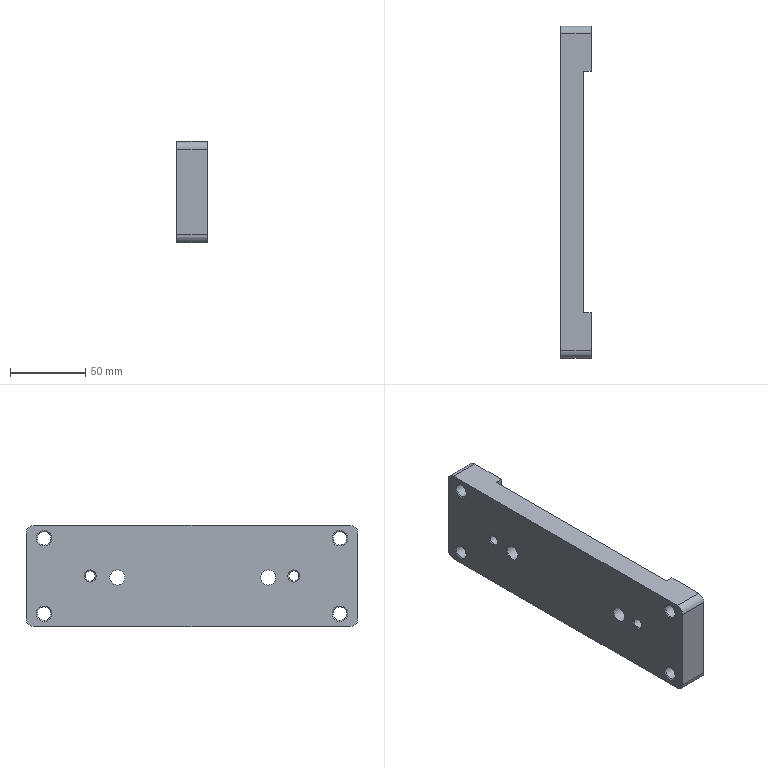Part | NX | features SIMPLE HOLE 8, DATUM_CSYS 6, SKETCH 5, HOLE PACKAGE 3, EXTRUDE 2, SYMBOLIC_THREAD 2, BLEND 1, LINKED_CURVE 1, LINKED_FACE 1 | 1 solid | 32 faces | box 20 x 220 x 67 mm | volume 232185 mm3 | cylinder 12 | plane 10 | cone 10 | commonest cylinder face diameters 10 x6 9 x4 6.8 x2
STEP:
#1=CARTESIAN_POINT('',(85.,105.,477.));
#2=VERTEX_POINT('',#1);
#3=CARTESIAN_POINT('',(85.,80.,477.));
#4=VERTEX_POINT('',#3);
#5=CARTESIAN_POINT('',(85.,110.,477.));
#6=DIRECTION('',(0.,-1.,0.));
#7=VECTOR('',#6,1000.);
#8=LINE('',#5,#7);
#9=EDGE_CURVE('',#2,#4,#8,.T.);
#10=ORIENTED_EDGE('',*,*,#9,.F.);
#11=CARTESIAN_POINT('',(65.,105.,477.));
#12=VERTEX_POINT('',#11);
#13=CARTESIAN_POINT('',(85.,105.,477.));
#14=DIRECTION('',(-1.,0.,0.));
#15=VECTOR('',#14,1000.);
#16=LINE('',#13,#15);
#17=EDGE_CURVE('',#2,#12,#16,.T.);
#18=ORIENTED_EDGE('',*,*,#17,.T.);
#19=CARTESIAN_POINT('',(65.,-105.,477.));
#20=VERTEX_POINT('',#19);
#21=CARTESIAN_POINT('',(65.,110.,477.));
#22=DIRECTION('',(0.,-1.,0.));
#23=VECTOR('',#22,1000.);
#24=LINE('',#21,#23);
#25=EDGE_CURVE('',#12,#20,#24,.T.);
#26=ORIENTED_EDGE('',*,*,#25,.T.);
#27=CARTESIAN_POINT('',(85.,-105.,477.));
#28=VERTEX_POINT('',#27);
#29=CARTESIAN_POINT('',(85.,-105.,477.));
#30=DIRECTION('',(-1.,0.,0.));
#31=VECTOR('',#30,1000.);
#32=LINE('',#29,#31);
#33=EDGE_CURVE('',#20,#28,#32,.F.);
#34=ORIENTED_EDGE('',*,*,#33,.T.);
#35=CARTESIAN_POINT('',(85.,-80.,477.));
#36=VERTEX_POINT('',#35);
#37=CARTESIAN_POINT('',(85.,110.,477.));
#38=DIRECTION('',(0.,-1.,0.));
#39=VECTOR('',#38,1000.);
#40=LINE('',#37,#39);
#41=EDGE_CURVE('',#36,#28,#40,.T.);
#42=ORIENTED_EDGE('',*,*,#41,.F.);
#43=CARTESIAN_POINT('',(80.,-80.,477.));
#44=VERTEX_POINT('',#43);
#45=CARTESIAN_POINT('',(80.,-80.,477.));
#46=DIRECTION('',(1.,0.,0.));
#47=VECTOR('',#46,1000.);
#48=LINE('',#45,#47);
#49=EDGE_CURVE('',#44,#36,#48,.T.);
#50=ORIENTED_EDGE('',*,*,#49,.F.);
#51=CARTESIAN_POINT('',(80.,80.,477.));
#52=VERTEX_POINT('',#51);
#53=CARTESIAN_POINT('',(80.,80.,477.));
#54=DIRECTION('',(0.,-1.,0.));
#55=VECTOR('',#54,1000.);
#56=LINE('',#53,#55);
#57=EDGE_CURVE('',#52,#44,#56,.T.);
#58=ORIENTED_EDGE('',*,*,#57,.F.);
#59=CARTESIAN_POINT('',(118.,80.,477.));
#60=DIRECTION('',(-1.,0.,0.));
#61=VECTOR('',#60,1000.);
#62=LINE('',#59,#61);
#63=EDGE_CURVE('',#4,#52,#62,.T.);
#64=ORIENTED_EDGE('',*,*,#63,.F.);
#65=EDGE_LOOP('',(#10,#18,#26,#34,#42,#50,#58,#64));
#66=FACE_BOUND('',#65,.T.);
#67=CARTESIAN_POINT('',(85.,110.,477.));
#68=DIRECTION('',(0.,0.,-1.));
#69=DIRECTION('',(0.,1.,0.));
#70=AXIS2_PLACEMENT_3D('',#67,#68,#69);
#71=PLANE('',#70);
#72=ADVANCED_FACE('',(#66),#71,.F.);
#73=CARTESIAN_POINT('',(85.,-98.,463.4));
#74=VERTEX_POINT('',#73);
#75=CARTESIAN_POINT('',(85.,-98.,468.5));
#76=DIRECTION('',(1.,0.,0.));
#77=DIRECTION('',(0.,0.,-1.));
#78=AXIS2_PLACEMENT_3D('',#75,#76,#77);
#79=CIRCLE('',#78,5.1);
#80=EDGE_CURVE('',#74,#74,#79,.F.);
#81=ORIENTED_EDGE('',*,*,#80,.T.);
#82=EDGE_LOOP('',(#81));
#83=FACE_BOUND('',#82,.T.);
#84=CARTESIAN_POINT('',(85.,-98.,413.4));
#85=VERTEX_POINT('',#84);
#86=CARTESIAN_POINT('',(85.,-98.,418.5));
#87=DIRECTION('',(1.,0.,0.));
#88=DIRECTION('',(0.,0.,-1.));
#89=AXIS2_PLACEMENT_3D('',#86,#87,#88);
#90=CIRCLE('',#89,5.1);
#91=EDGE_CURVE('',#85,#85,#90,.F.);
#92=ORIENTED_EDGE('',*,*,#91,.T.);
#93=EDGE_LOOP('',(#92));
#94=FACE_BOUND('',#93,.T.);
#95=CARTESIAN_POINT('',(85.,-110.,472.));
#96=VERTEX_POINT('',#95);
#97=CARTESIAN_POINT('',(85.,-110.,415.));
#98=VERTEX_POINT('',#97);
#99=CARTESIAN_POINT('',(85.,-110.,477.));
#100=DIRECTION('',(0.,0.,-1.));
#101=VECTOR('',#100,1000.);
#102=LINE('',#99,#101);
#103=EDGE_CURVE('',#96,#98,#102,.T.);
#104=ORIENTED_EDGE('',*,*,#103,.T.);
#105=CARTESIAN_POINT('',(85.,-105.,410.));
#106=VERTEX_POINT('',#105);
#107=CARTESIAN_POINT('',(85.,-105.,415.));
#108=DIRECTION('',(1.,0.,0.));
#109=DIRECTION('',(0.,0.,-1.));
#110=AXIS2_PLACEMENT_3D('',#107,#108,#109);
#111=CIRCLE('',#110,5.);
#112=EDGE_CURVE('',#98,#106,#111,.T.);
#113=ORIENTED_EDGE('',*,*,#112,.T.);
#114=CARTESIAN_POINT('',(85.,-80.,410.));
#115=VERTEX_POINT('',#114);
#116=CARTESIAN_POINT('',(85.,-110.,410.));
#117=DIRECTION('',(0.,1.,0.));
#118=VECTOR('',#117,1000.);
#119=LINE('',#116,#118);
#120=EDGE_CURVE('',#106,#115,#119,.T.);
#121=ORIENTED_EDGE('',*,*,#120,.T.);
#122=CARTESIAN_POINT('',(85.,-80.,0.));
#123=DIRECTION('',(0.,0.,-1.));
#124=VECTOR('',#123,1000.);
#125=LINE('',#122,#124);
#126=EDGE_CURVE('',#36,#115,#125,.T.);
#127=ORIENTED_EDGE('',*,*,#126,.F.);
#128=ORIENTED_EDGE('',*,*,#41,.T.);
#129=CARTESIAN_POINT('',(85.,-105.,472.));
#130=DIRECTION('',(1.,0.,0.));
#131=DIRECTION('',(0.,0.,-1.));
#132=AXIS2_PLACEMENT_3D('',#129,#130,#131);
#133=CIRCLE('',#132,5.);
#134=EDGE_CURVE('',#28,#96,#133,.T.);
#135=ORIENTED_EDGE('',*,*,#134,.T.);
#136=EDGE_LOOP('',(#104,#113,#121,#127,#128,#135));
#137=FACE_BOUND('',#136,.T.);
#138=CARTESIAN_POINT('',(85.,0.,0.));
#139=DIRECTION('',(1.,0.,0.));
#140=DIRECTION('',(0.,0.,-1.));
#141=AXIS2_PLACEMENT_3D('',#138,#139,#140);
#142=PLANE('',#141);
#143=ADVANCED_FACE('',(#83,#94,#137),#142,.T.);
#144=CARTESIAN_POINT('',(65.,-110.,472.));
#145=VERTEX_POINT('',#144);
#146=CARTESIAN_POINT('',(65.,-110.,415.));
#147=VERTEX_POINT('',#146);
#148=CARTESIAN_POINT('',(65.,-110.,477.));
#149=DIRECTION('',(0.,0.,-1.));
#150=VECTOR('',#149,1000.);
#151=LINE('',#148,#150);
#152=EDGE_CURVE('',#145,#147,#151,.T.);
#153=ORIENTED_EDGE('',*,*,#152,.T.);
#154=CARTESIAN_POINT('',(85.,-110.,415.));
#155=DIRECTION('',(-1.,0.,0.));
#156=VECTOR('',#155,1000.);
#157=LINE('',#154,#156);
#158=EDGE_CURVE('',#147,#98,#157,.F.);
#159=ORIENTED_EDGE('',*,*,#158,.T.);
#160=ORIENTED_EDGE('',*,*,#103,.F.);
#161=CARTESIAN_POINT('',(85.,-110.,472.));
#162=DIRECTION('',(-1.,0.,0.));
#163=VECTOR('',#162,1000.);
#164=LINE('',#161,#163);
#165=EDGE_CURVE('',#96,#145,#164,.T.);
#166=ORIENTED_EDGE('',*,*,#165,.T.);
#167=EDGE_LOOP('',(#153,#159,#160,#166));
#168=FACE_BOUND('',#167,.T.);
#169=CARTESIAN_POINT('',(85.,-110.,477.));
#170=DIRECTION('',(0.,1.,0.));
#171=DIRECTION('',(0.,0.,1.));
#172=AXIS2_PLACEMENT_3D('',#169,#170,#171);
#173=PLANE('',#172);
#174=ADVANCED_FACE('',(#168),#173,.F.);
#175=CARTESIAN_POINT('',(65.,-105.,410.));
#176=VERTEX_POINT('',#175);
#177=CARTESIAN_POINT('',(65.,105.,410.));
#178=VERTEX_POINT('',#177);
#179=CARTESIAN_POINT('',(65.,-110.,410.));
#180=DIRECTION('',(0.,1.,0.));
#181=VECTOR('',#180,1000.);
#182=LINE('',#179,#181);
#183=EDGE_CURVE('',#176,#178,#182,.T.);
#184=ORIENTED_EDGE('',*,*,#183,.T.);
#185=CARTESIAN_POINT('',(85.,105.,410.));
#186=VERTEX_POINT('',#185);
#187=CARTESIAN_POINT('',(85.,105.,410.));
#188=DIRECTION('',(-1.,0.,0.));
#189=VECTOR('',#188,1000.);
#190=LINE('',#187,#189);
#191=EDGE_CURVE('',#178,#186,#190,.F.);
#192=ORIENTED_EDGE('',*,*,#191,.T.);
#193=CARTESIAN_POINT('',(85.,80.,410.));
#194=VERTEX_POINT('',#193);
#195=CARTESIAN_POINT('',(85.,-110.,410.));
#196=DIRECTION('',(0.,1.,0.));
#197=VECTOR('',#196,1000.);
#198=LINE('',#195,#197);
#199=EDGE_CURVE('',#194,#186,#198,.T.);
#200=ORIENTED_EDGE('',*,*,#199,.F.);
#201=CARTESIAN_POINT('',(80.,80.,410.));
#202=VERTEX_POINT('',#201);
#203=CARTESIAN_POINT('',(85.,80.,410.));
#204=DIRECTION('',(-1.,0.,0.));
#205=VECTOR('',#204,1000.);
#206=LINE('',#203,#205);
#207=EDGE_CURVE('',#194,#202,#206,.T.);
#208=ORIENTED_EDGE('',*,*,#207,.T.);
#209=CARTESIAN_POINT('',(80.,-80.,410.));
#210=VERTEX_POINT('',#209);
#211=CARTESIAN_POINT('',(80.,-110.,410.));
#212=DIRECTION('',(0.,-1.,0.));
#213=VECTOR('',#212,1000.);
#214=LINE('',#211,#213);
#215=EDGE_CURVE('',#202,#210,#214,.T.);
#216=ORIENTED_EDGE('',*,*,#215,.T.);
#217=CARTESIAN_POINT('',(85.,-80.,410.));
#218=DIRECTION('',(1.,0.,0.));
#219=VECTOR('',#218,1000.);
#220=LINE('',#217,#219);
#221=EDGE_CURVE('',#210,#115,#220,.T.);
#222=ORIENTED_EDGE('',*,*,#221,.T.);
#223=ORIENTED_EDGE('',*,*,#120,.F.);
#224=CARTESIAN_POINT('',(85.,-105.,410.));
#225=DIRECTION('',(-1.,0.,0.));
#226=VECTOR('',#225,1000.);
#227=LINE('',#224,#226);
#228=EDGE_CURVE('',#106,#176,#227,.T.);
#229=ORIENTED_EDGE('',*,*,#228,.T.);
#230=EDGE_LOOP('',(#184,#192,#200,#208,#216,#222,#223,#229));
#231=FACE_BOUND('',#230,.T.);
#232=CARTESIAN_POINT('',(85.,-110.,410.));
#233=DIRECTION('',(0.,0.,1.));
#234=DIRECTION('',(1.,0.,0.));
#235=AXIS2_PLACEMENT_3D('',#232,#233,#234);
#236=PLANE('',#235);
#237=ADVANCED_FACE('',(#231),#236,.F.);
#238=CARTESIAN_POINT('',(85.,110.,415.));
#239=VERTEX_POINT('',#238);
#240=CARTESIAN_POINT('',(85.,110.,472.));
#241=VERTEX_POINT('',#240);
#242=CARTESIAN_POINT('',(85.,110.,410.));
#243=DIRECTION('',(0.,0.,1.));
#244=VECTOR('',#243,1000.);
#245=LINE('',#242,#244);
#246=EDGE_CURVE('',#239,#241,#245,.T.);
#247=ORIENTED_EDGE('',*,*,#246,.F.);
#248=CARTESIAN_POINT('',(65.,110.,415.));
#249=VERTEX_POINT('',#248);
#250=CARTESIAN_POINT('',(85.,110.,415.));
#251=DIRECTION('',(-1.,0.,0.));
#252=VECTOR('',#251,1000.);
#253=LINE('',#250,#252);
#254=EDGE_CURVE('',#239,#249,#253,.T.);
#255=ORIENTED_EDGE('',*,*,#254,.T.);
#256=CARTESIAN_POINT('',(65.,110.,472.));
#257=VERTEX_POINT('',#256);
#258=CARTESIAN_POINT('',(65.,110.,410.));
#259=DIRECTION('',(0.,0.,1.));
#260=VECTOR('',#259,1000.);
#261=LINE('',#258,#260);
#262=EDGE_CURVE('',#249,#257,#261,.T.);
#263=ORIENTED_EDGE('',*,*,#262,.T.);
#264=CARTESIAN_POINT('',(85.,110.,472.));
#265=DIRECTION('',(-1.,0.,0.));
#266=VECTOR('',#265,1000.);
#267=LINE('',#264,#266);
#268=EDGE_CURVE('',#257,#241,#267,.F.);
#269=ORIENTED_EDGE('',*,*,#268,.T.);
#270=EDGE_LOOP('',(#247,#255,#263,#269));
#271=FACE_BOUND('',#270,.T.);
#272=CARTESIAN_POINT('',(85.,110.,410.));
#273=DIRECTION('',(0.,-1.,0.));
#274=DIRECTION('',(0.,0.,-1.));
#275=AXIS2_PLACEMENT_3D('',#272,#273,#274);
#276=PLANE('',#275);
#277=ADVANCED_FACE('',(#271),#276,.F.);
#278=CARTESIAN_POINT('',(85.,98.,463.4));
#279=VERTEX_POINT('',#278);
#280=CARTESIAN_POINT('',(85.,98.,468.5));
#281=DIRECTION('',(1.,0.,0.));
#282=DIRECTION('',(0.,0.,-1.));
#283=AXIS2_PLACEMENT_3D('',#280,#281,#282);
#284=CIRCLE('',#283,5.1);
#285=EDGE_CURVE('',#279,#279,#284,.F.);
#286=ORIENTED_EDGE('',*,*,#285,.T.);
#287=EDGE_LOOP('',(#286));
#288=FACE_BOUND('',#287,.T.);
#289=CARTESIAN_POINT('',(85.,98.,413.4));
#290=VERTEX_POINT('',#289);
#291=CARTESIAN_POINT('',(85.,98.,418.5));
#292=DIRECTION('',(1.,0.,0.));
#293=DIRECTION('',(0.,0.,-1.));
#294=AXIS2_PLACEMENT_3D('',#291,#292,#293);
#295=CIRCLE('',#294,5.1);
#296=EDGE_CURVE('',#290,#290,#295,.F.);
#297=ORIENTED_EDGE('',*,*,#296,.T.);
#298=EDGE_LOOP('',(#297));
#299=FACE_BOUND('',#298,.T.);
#300=ORIENTED_EDGE('',*,*,#199,.T.);
#301=CARTESIAN_POINT('',(85.,105.,415.));
#302=DIRECTION('',(1.,0.,0.));
#303=DIRECTION('',(0.,0.,-1.));
#304=AXIS2_PLACEMENT_3D('',#301,#302,#303);
#305=CIRCLE('',#304,5.);
#306=EDGE_CURVE('',#186,#239,#305,.T.);
#307=ORIENTED_EDGE('',*,*,#306,.T.);
#308=ORIENTED_EDGE('',*,*,#246,.T.);
#309=CARTESIAN_POINT('',(85.,105.,472.));
#310=DIRECTION('',(1.,0.,0.));
#311=DIRECTION('',(0.,0.,-1.));
#312=AXIS2_PLACEMENT_3D('',#309,#310,#311);
#313=CIRCLE('',#312,5.);
#314=EDGE_CURVE('',#241,#2,#313,.T.);
#315=ORIENTED_EDGE('',*,*,#314,.T.);
#316=ORIENTED_EDGE('',*,*,#9,.T.);
#317=CARTESIAN_POINT('',(85.,80.,0.));
#318=DIRECTION('',(0.,0.,1.));
#319=VECTOR('',#318,1000.);
#320=LINE('',#317,#319);
#321=EDGE_CURVE('',#194,#4,#320,.T.);
#322=ORIENTED_EDGE('',*,*,#321,.F.);
#323=EDGE_LOOP('',(#300,#307,#308,#315,#316,#322));
#324=FACE_BOUND('',#323,.T.);
#325=CARTESIAN_POINT('',(85.,0.,0.));
#326=DIRECTION('',(1.,0.,0.));
#327=DIRECTION('',(0.,0.,-1.));
#328=AXIS2_PLACEMENT_3D('',#325,#326,#327);
#329=PLANE('',#328);
#330=ADVANCED_FACE('',(#288,#299,#324),#329,.T.);
#331=CARTESIAN_POINT('',(65.,98.,463.4));
#332=VERTEX_POINT('',#331);
#333=CARTESIAN_POINT('',(65.,98.,468.5));
#334=DIRECTION('',(1.,0.,0.));
#335=DIRECTION('',(0.,0.,-1.));
#336=AXIS2_PLACEMENT_3D('',#333,#334,#335);
#337=CIRCLE('',#336,5.1);
#338=EDGE_CURVE('',#332,#332,#337,.T.);
#339=ORIENTED_EDGE('',*,*,#338,.T.);
#340=EDGE_LOOP('',(#339));
#341=FACE_BOUND('',#340,.T.);
#342=CARTESIAN_POINT('',(65.,98.,413.4));
#343=VERTEX_POINT('',#342);
#344=CARTESIAN_POINT('',(65.,98.,418.5));
#345=DIRECTION('',(1.,0.,0.));
#346=DIRECTION('',(0.,0.,-1.));
#347=AXIS2_PLACEMENT_3D('',#344,#345,#346);
#348=CIRCLE('',#347,5.1);
#349=EDGE_CURVE('',#343,#343,#348,.T.);
#350=ORIENTED_EDGE('',*,*,#349,.T.);
#351=EDGE_LOOP('',(#350));
#352=FACE_BOUND('',#351,.T.);
#353=CARTESIAN_POINT('',(65.,-98.,463.4));
#354=VERTEX_POINT('',#353);
#355=CARTESIAN_POINT('',(65.,-98.,468.5));
#356=DIRECTION('',(1.,0.,0.));
#357=DIRECTION('',(0.,0.,-1.));
#358=AXIS2_PLACEMENT_3D('',#355,#356,#357);
#359=CIRCLE('',#358,5.1);
#360=EDGE_CURVE('',#354,#354,#359,.T.);
#361=ORIENTED_EDGE('',*,*,#360,.T.);
#362=EDGE_LOOP('',(#361));
#363=FACE_BOUND('',#362,.T.);
#364=CARTESIAN_POINT('',(65.,-98.,413.4));
#365=VERTEX_POINT('',#364);
#366=CARTESIAN_POINT('',(65.,-98.,418.5));
#367=DIRECTION('',(1.,0.,0.));
#368=DIRECTION('',(0.,0.,-1.));
#369=AXIS2_PLACEMENT_3D('',#366,#367,#368);
#370=CIRCLE('',#369,5.1);
#371=EDGE_CURVE('',#365,#365,#370,.T.);
#372=ORIENTED_EDGE('',*,*,#371,.T.);
#373=EDGE_LOOP('',(#372));
#374=FACE_BOUND('',#373,.T.);
#375=CARTESIAN_POINT('',(65.,-50.5,437.5));
#376=VERTEX_POINT('',#375);
#377=CARTESIAN_POINT('',(65.,-50.5,442.5));
#378=DIRECTION('',(1.,0.,0.));
#379=DIRECTION('',(0.,0.,-1.));
#380=AXIS2_PLACEMENT_3D('',#377,#378,#379);
#381=CIRCLE('',#380,5.);
#382=EDGE_CURVE('',#376,#376,#381,.T.);
#383=ORIENTED_EDGE('',*,*,#382,.T.);
#384=EDGE_LOOP('',(#383));
#385=FACE_BOUND('',#384,.T.);
#386=CARTESIAN_POINT('',(65.,49.5,437.5));
#387=VERTEX_POINT('',#386);
#388=CARTESIAN_POINT('',(65.,49.5,442.5));
#389=DIRECTION('',(1.,0.,0.));
#390=DIRECTION('',(0.,0.,-1.));
#391=AXIS2_PLACEMENT_3D('',#388,#389,#390);
#392=CIRCLE('',#391,5.);
#393=EDGE_CURVE('',#387,#387,#392,.T.);
#394=ORIENTED_EDGE('',*,*,#393,.T.);
#395=EDGE_LOOP('',(#394));
#396=FACE_BOUND('',#395,.T.);
#397=CARTESIAN_POINT('',(65.,67.5,439.5));
#398=VERTEX_POINT('',#397);
#399=CARTESIAN_POINT('',(65.,67.5,443.5));
#400=DIRECTION('',(1.,0.,0.));
#401=DIRECTION('',(0.,0.,-1.));
#402=AXIS2_PLACEMENT_3D('',#399,#400,#401);
#403=CIRCLE('',#402,4.);
#404=EDGE_CURVE('',#398,#398,#403,.T.);
#405=ORIENTED_EDGE('',*,*,#404,.T.);
#406=EDGE_LOOP('',(#405));
#407=FACE_BOUND('',#406,.T.);
#408=CARTESIAN_POINT('',(65.,-67.5,439.5));
#409=VERTEX_POINT('',#408);
#410=CARTESIAN_POINT('',(65.,-67.5,443.5));
#411=DIRECTION('',(1.,0.,0.));
#412=DIRECTION('',(0.,0.,-1.));
#413=AXIS2_PLACEMENT_3D('',#410,#411,#412);
#414=CIRCLE('',#413,4.);
#415=EDGE_CURVE('',#409,#409,#414,.T.);
#416=ORIENTED_EDGE('',*,*,#415,.T.);
#417=EDGE_LOOP('',(#416));
#418=FACE_BOUND('',#417,.T.);
#419=ORIENTED_EDGE('',*,*,#262,.F.);
#420=CARTESIAN_POINT('',(65.,105.,415.));
#421=DIRECTION('',(1.,0.,0.));
#422=DIRECTION('',(0.,0.,-1.));
#423=AXIS2_PLACEMENT_3D('',#420,#421,#422);
#424=CIRCLE('',#423,5.);
#425=EDGE_CURVE('',#249,#178,#424,.F.);
#426=ORIENTED_EDGE('',*,*,#425,.T.);
#427=ORIENTED_EDGE('',*,*,#183,.F.);
#428=CARTESIAN_POINT('',(65.,-105.,415.));
#429=DIRECTION('',(1.,0.,0.));
#430=DIRECTION('',(0.,0.,-1.));
#431=AXIS2_PLACEMENT_3D('',#428,#429,#430);
#432=CIRCLE('',#431,5.);
#433=EDGE_CURVE('',#176,#147,#432,.F.);
#434=ORIENTED_EDGE('',*,*,#433,.T.);
#435=ORIENTED_EDGE('',*,*,#152,.F.);
#436=CARTESIAN_POINT('',(65.,-105.,472.));
#437=DIRECTION('',(1.,0.,0.));
#438=DIRECTION('',(0.,0.,-1.));
#439=AXIS2_PLACEMENT_3D('',#436,#437,#438);
#440=CIRCLE('',#439,5.);
#441=EDGE_CURVE('',#145,#20,#440,.F.);
#442=ORIENTED_EDGE('',*,*,#441,.T.);
#443=ORIENTED_EDGE('',*,*,#25,.F.);
#444=CARTESIAN_POINT('',(65.,105.,472.));
#445=DIRECTION('',(1.,0.,0.));
#446=DIRECTION('',(0.,0.,-1.));
#447=AXIS2_PLACEMENT_3D('',#444,#445,#446);
#448=CIRCLE('',#447,5.);
#449=EDGE_CURVE('',#12,#257,#448,.F.);
#450=ORIENTED_EDGE('',*,*,#449,.T.);
#451=EDGE_LOOP('',(#419,#426,#427,#434,#435,#442,#443,#450));
#452=FACE_BOUND('',#451,.T.);
#453=CARTESIAN_POINT('',(65.,0.,0.));
#454=DIRECTION('',(1.,0.,0.));
#455=DIRECTION('',(0.,0.,-1.));
#456=AXIS2_PLACEMENT_3D('',#453,#454,#455);
#457=PLANE('',#456);
#458=ADVANCED_FACE('',(#341,#352,#363,#374,#385,#396,#407,#418,#452),#457,.F.);
#459=CARTESIAN_POINT('',(80.,-67.5,446.9));
#460=VERTEX_POINT('',#459);
#461=CARTESIAN_POINT('',(80.,-67.5,443.5));
#462=DIRECTION('',(-1.,0.,0.));
#463=DIRECTION('',(0.,0.,1.));
#464=AXIS2_PLACEMENT_3D('',#461,#462,#463);
#465=CIRCLE('',#464,3.4);
#466=EDGE_CURVE('',#460,#460,#465,.F.);
#467=ORIENTED_EDGE('',*,*,#466,.T.);
#468=EDGE_LOOP('',(#467));
#469=FACE_BOUND('',#468,.T.);
#470=CARTESIAN_POINT('',(65.6,-67.5,440.1));
#471=VERTEX_POINT('',#470);
#472=CARTESIAN_POINT('',(65.6,-67.5,443.5));
#473=DIRECTION('',(1.,0.,0.));
#474=DIRECTION('',(0.,0.,-1.));
#475=AXIS2_PLACEMENT_3D('',#472,#473,#474);
#476=CIRCLE('',#475,3.4);
#477=EDGE_CURVE('',#471,#471,#476,.F.);
#478=ORIENTED_EDGE('',*,*,#477,.T.);
#479=EDGE_LOOP('',(#478));
#480=FACE_BOUND('',#479,.T.);
#481=CARTESIAN_POINT('',(65.,-67.5,443.5));
#482=DIRECTION('',(1.,0.,0.));
#483=DIRECTION('',(0.,0.,-1.));
#484=AXIS2_PLACEMENT_3D('',#481,#482,#483);
#485=CYLINDRICAL_SURFACE('',#484,3.4);
#486=ADVANCED_FACE('',(#469,#480),#485,.F.);
#487=ORIENTED_EDGE('',*,*,#477,.F.);
#488=EDGE_LOOP('',(#487));
#489=FACE_BOUND('',#488,.T.);
#490=ORIENTED_EDGE('',*,*,#415,.F.);
#491=EDGE_LOOP('',(#490));
#492=FACE_BOUND('',#491,.T.);
#493=CARTESIAN_POINT('',(65.,-67.5,443.5));
#494=DIRECTION('',(-1.,0.,0.));
#495=DIRECTION('',(0.,0.,1.));
#496=AXIS2_PLACEMENT_3D('',#493,#494,#495);
#497=CONICAL_SURFACE('',#496,4.,0.7854);
#498=ADVANCED_FACE('',(#489,#492),#497,.F.);
#499=CARTESIAN_POINT('',(80.,67.5,446.9));
#500=VERTEX_POINT('',#499);
#501=CARTESIAN_POINT('',(80.,67.5,443.5));
#502=DIRECTION('',(-1.,0.,0.));
#503=DIRECTION('',(0.,0.,1.));
#504=AXIS2_PLACEMENT_3D('',#501,#502,#503);
#505=CIRCLE('',#504,3.4);
#506=EDGE_CURVE('',#500,#500,#505,.F.);
#507=ORIENTED_EDGE('',*,*,#506,.T.);
#508=EDGE_LOOP('',(#507));
#509=FACE_BOUND('',#508,.T.);
#510=CARTESIAN_POINT('',(65.6,67.5,440.1));
#511=VERTEX_POINT('',#510);
#512=CARTESIAN_POINT('',(65.6,67.5,443.5));
#513=DIRECTION('',(1.,0.,0.));
#514=DIRECTION('',(0.,0.,-1.));
#515=AXIS2_PLACEMENT_3D('',#512,#513,#514);
#516=CIRCLE('',#515,3.4);
#517=EDGE_CURVE('',#511,#511,#516,.F.);
#518=ORIENTED_EDGE('',*,*,#517,.T.);
#519=EDGE_LOOP('',(#518));
#520=FACE_BOUND('',#519,.T.);
#521=CARTESIAN_POINT('',(65.,67.5,443.5));
#522=DIRECTION('',(1.,0.,0.));
#523=DIRECTION('',(0.,0.,-1.));
#524=AXIS2_PLACEMENT_3D('',#521,#522,#523);
#525=CYLINDRICAL_SURFACE('',#524,3.4);
#526=ADVANCED_FACE('',(#509,#520),#525,.F.);
#527=ORIENTED_EDGE('',*,*,#517,.F.);
#528=EDGE_LOOP('',(#527));
#529=FACE_BOUND('',#528,.T.);
#530=ORIENTED_EDGE('',*,*,#404,.F.);
#531=EDGE_LOOP('',(#530));
#532=FACE_BOUND('',#531,.T.);
#533=CARTESIAN_POINT('',(65.,67.5,443.5));
#534=DIRECTION('',(-1.,0.,0.));
#535=DIRECTION('',(0.,0.,1.));
#536=AXIS2_PLACEMENT_3D('',#533,#534,#535);
#537=CONICAL_SURFACE('',#536,4.,0.7854);
#538=ADVANCED_FACE('',(#529,#532),#537,.F.);
#539=CARTESIAN_POINT('',(80.,-80.,402.));
#540=DIRECTION('',(0.,0.,1.));
#541=VECTOR('',#540,1000.);
#542=LINE('',#539,#541);
#543=EDGE_CURVE('',#44,#210,#542,.F.);
#544=ORIENTED_EDGE('',*,*,#543,.F.);
#545=ORIENTED_EDGE('',*,*,#49,.T.);
#546=ORIENTED_EDGE('',*,*,#126,.T.);
#547=ORIENTED_EDGE('',*,*,#221,.F.);
#548=EDGE_LOOP('',(#544,#545,#546,#547));
#549=FACE_BOUND('',#548,.T.);
#550=CARTESIAN_POINT('',(80.,-80.,402.));
#551=DIRECTION('',(0.,-1.,0.));
#552=DIRECTION('',(0.,0.,-1.));
#553=AXIS2_PLACEMENT_3D('',#550,#551,#552);
#554=PLANE('',#553);
#555=ADVANCED_FACE('',(#549),#554,.F.);
#556=ORIENTED_EDGE('',*,*,#321,.T.);
#557=ORIENTED_EDGE('',*,*,#63,.T.);
#558=CARTESIAN_POINT('',(80.,80.,402.));
#559=DIRECTION('',(0.,0.,1.));
#560=VECTOR('',#559,1000.);
#561=LINE('',#558,#560);
#562=EDGE_CURVE('',#52,#202,#561,.F.);
#563=ORIENTED_EDGE('',*,*,#562,.T.);
#564=ORIENTED_EDGE('',*,*,#207,.F.);
#565=EDGE_LOOP('',(#556,#557,#563,#564));
#566=FACE_BOUND('',#565,.T.);
#567=CARTESIAN_POINT('',(118.,80.,402.));
#568=DIRECTION('',(0.,1.,0.));
#569=DIRECTION('',(0.,0.,1.));
#570=AXIS2_PLACEMENT_3D('',#567,#568,#569);
#571=PLANE('',#570);
#572=ADVANCED_FACE('',(#566),#571,.F.);
#573=CARTESIAN_POINT('',(80.,-50.5,447.5));
#574=VERTEX_POINT('',#573);
#575=CARTESIAN_POINT('',(80.,-50.5,442.5));
#576=DIRECTION('',(-1.,0.,0.));
#577=DIRECTION('',(0.,0.,1.));
#578=AXIS2_PLACEMENT_3D('',#575,#576,#577);
#579=CIRCLE('',#578,5.);
#580=EDGE_CURVE('',#574,#574,#579,.T.);
#581=ORIENTED_EDGE('',*,*,#580,.T.);
#582=EDGE_LOOP('',(#581));
#583=FACE_BOUND('',#582,.T.);
#584=CARTESIAN_POINT('',(80.,49.5,447.5));
#585=VERTEX_POINT('',#584);
#586=CARTESIAN_POINT('',(80.,49.5,442.5));
#587=DIRECTION('',(-1.,0.,0.));
#588=DIRECTION('',(0.,0.,1.));
#589=AXIS2_PLACEMENT_3D('',#586,#587,#588);
#590=CIRCLE('',#589,5.);
#591=EDGE_CURVE('',#585,#585,#590,.T.);
#592=ORIENTED_EDGE('',*,*,#591,.T.);
#593=EDGE_LOOP('',(#592));
#594=FACE_BOUND('',#593,.T.);
#595=ORIENTED_EDGE('',*,*,#506,.F.);
#596=EDGE_LOOP('',(#595));
#597=FACE_BOUND('',#596,.T.);
#598=ORIENTED_EDGE('',*,*,#466,.F.);
#599=EDGE_LOOP('',(#598));
#600=FACE_BOUND('',#599,.T.);
#601=ORIENTED_EDGE('',*,*,#562,.F.);
#602=ORIENTED_EDGE('',*,*,#57,.T.);
#603=ORIENTED_EDGE('',*,*,#543,.T.);
#604=ORIENTED_EDGE('',*,*,#215,.F.);
#605=EDGE_LOOP('',(#601,#602,#603,#604));
#606=FACE_BOUND('',#605,.T.);
#607=CARTESIAN_POINT('',(80.,80.,402.));
#608=DIRECTION('',(-1.,0.,0.));
#609=DIRECTION('',(0.,0.,1.));
#610=AXIS2_PLACEMENT_3D('',#607,#608,#609);
#611=PLANE('',#610);
#612=ADVANCED_FACE('',(#583,#594,#597,#600,#606),#611,.F.);
#613=ORIENTED_EDGE('',*,*,#306,.F.);
#614=ORIENTED_EDGE('',*,*,#191,.F.);
#615=ORIENTED_EDGE('',*,*,#425,.F.);
#616=ORIENTED_EDGE('',*,*,#254,.F.);
#617=EDGE_LOOP('',(#613,#614,#615,#616));
#618=FACE_BOUND('',#617,.T.);
#619=CARTESIAN_POINT('',(85.,105.,415.));
#620=DIRECTION('',(-1.,0.,0.));
#621=DIRECTION('',(0.,0.,1.));
#622=AXIS2_PLACEMENT_3D('',#619,#620,#621);
#623=CYLINDRICAL_SURFACE('',#622,5.);
#624=ADVANCED_FACE('',(#618),#623,.T.);
#625=ORIENTED_EDGE('',*,*,#314,.F.);
#626=ORIENTED_EDGE('',*,*,#268,.F.);
#627=ORIENTED_EDGE('',*,*,#449,.F.);
#628=ORIENTED_EDGE('',*,*,#17,.F.);
#629=EDGE_LOOP('',(#625,#626,#627,#628));
#630=FACE_BOUND('',#629,.T.);
#631=CARTESIAN_POINT('',(85.,105.,472.));
#632=DIRECTION('',(-1.,0.,0.));
#633=DIRECTION('',(0.,0.,1.));
#634=AXIS2_PLACEMENT_3D('',#631,#632,#633);
#635=CYLINDRICAL_SURFACE('',#634,5.);
#636=ADVANCED_FACE('',(#630),#635,.T.);
#637=ORIENTED_EDGE('',*,*,#112,.F.);
#638=ORIENTED_EDGE('',*,*,#158,.F.);
#639=ORIENTED_EDGE('',*,*,#433,.F.);
#640=ORIENTED_EDGE('',*,*,#228,.F.);
#641=EDGE_LOOP('',(#637,#638,#639,#640));
#642=FACE_BOUND('',#641,.T.);
#643=CARTESIAN_POINT('',(85.,-105.,415.));
#644=DIRECTION('',(-1.,0.,0.));
#645=DIRECTION('',(0.,0.,1.));
#646=AXIS2_PLACEMENT_3D('',#643,#644,#645);
#647=CYLINDRICAL_SURFACE('',#646,5.);
#648=ADVANCED_FACE('',(#642),#647,.T.);
#649=ORIENTED_EDGE('',*,*,#134,.F.);
#650=ORIENTED_EDGE('',*,*,#33,.F.);
#651=ORIENTED_EDGE('',*,*,#441,.F.);
#652=ORIENTED_EDGE('',*,*,#165,.F.);
#653=EDGE_LOOP('',(#649,#650,#651,#652));
#654=FACE_BOUND('',#653,.T.);
#655=CARTESIAN_POINT('',(85.,-105.,472.));
#656=DIRECTION('',(-1.,0.,0.));
#657=DIRECTION('',(0.,0.,1.));
#658=AXIS2_PLACEMENT_3D('',#655,#656,#657);
#659=CYLINDRICAL_SURFACE('',#658,5.);
#660=ADVANCED_FACE('',(#654),#659,.T.);
#661=ORIENTED_EDGE('',*,*,#393,.F.);
#662=EDGE_LOOP('',(#661));
#663=FACE_BOUND('',#662,.T.);
#664=ORIENTED_EDGE('',*,*,#591,.F.);
#665=EDGE_LOOP('',(#664));
#666=FACE_BOUND('',#665,.T.);
#667=CARTESIAN_POINT('',(65.,49.5,442.5));
#668=DIRECTION('',(1.,0.,0.));
#669=DIRECTION('',(0.,0.,-1.));
#670=AXIS2_PLACEMENT_3D('',#667,#668,#669);
#671=CYLINDRICAL_SURFACE('',#670,5.);
#672=ADVANCED_FACE('',(#663,#666),#671,.F.);
#673=ORIENTED_EDGE('',*,*,#382,.F.);
#674=EDGE_LOOP('',(#673));
#675=FACE_BOUND('',#674,.T.);
#676=ORIENTED_EDGE('',*,*,#580,.F.);
#677=EDGE_LOOP('',(#676));
#678=FACE_BOUND('',#677,.T.);
#679=CARTESIAN_POINT('',(65.,-50.5,442.5));
#680=DIRECTION('',(1.,0.,0.));
#681=DIRECTION('',(0.,0.,-1.));
#682=AXIS2_PLACEMENT_3D('',#679,#680,#681);
#683=CYLINDRICAL_SURFACE('',#682,5.);
#684=ADVANCED_FACE('',(#675,#678),#683,.F.);
#685=CARTESIAN_POINT('',(84.4,-98.,414.));
#686=VERTEX_POINT('',#685);
#687=CARTESIAN_POINT('',(84.4,-98.,418.5));
#688=DIRECTION('',(1.,0.,0.));
#689=DIRECTION('',(0.,0.,-1.));
#690=AXIS2_PLACEMENT_3D('',#687,#688,#689);
#691=CIRCLE('',#690,4.5);
#692=EDGE_CURVE('',#686,#686,#691,.T.);
#693=ORIENTED_EDGE('',*,*,#692,.T.);
#694=EDGE_LOOP('',(#693));
#695=FACE_BOUND('',#694,.T.);
#696=CARTESIAN_POINT('',(65.6,-98.,414.));
#697=VERTEX_POINT('',#696);
#698=CARTESIAN_POINT('',(65.6,-98.,418.5));
#699=DIRECTION('',(1.,0.,0.));
#700=DIRECTION('',(0.,0.,-1.));
#701=AXIS2_PLACEMENT_3D('',#698,#699,#700);
#702=CIRCLE('',#701,4.5);
#703=EDGE_CURVE('',#697,#697,#702,.F.);
#704=ORIENTED_EDGE('',*,*,#703,.T.);
#705=EDGE_LOOP('',(#704));
#706=FACE_BOUND('',#705,.T.);
#707=CARTESIAN_POINT('',(65.,-98.,418.5));
#708=DIRECTION('',(1.,0.,0.));
#709=DIRECTION('',(0.,0.,-1.));
#710=AXIS2_PLACEMENT_3D('',#707,#708,#709);
#711=CYLINDRICAL_SURFACE('',#710,4.5);
#712=ADVANCED_FACE('',(#695,#706),#711,.F.);
#713=ORIENTED_EDGE('',*,*,#703,.F.);
#714=EDGE_LOOP('',(#713));
#715=FACE_BOUND('',#714,.T.);
#716=ORIENTED_EDGE('',*,*,#371,.F.);
#717=EDGE_LOOP('',(#716));
#718=FACE_BOUND('',#717,.T.);
#719=CARTESIAN_POINT('',(65.,-98.,418.5));
#720=DIRECTION('',(-1.,0.,0.));
#721=DIRECTION('',(0.,0.,1.));
#722=AXIS2_PLACEMENT_3D('',#719,#720,#721);
#723=CONICAL_SURFACE('',#722,5.1,0.7854);
#724=ADVANCED_FACE('',(#715,#718),#723,.F.);
#725=ORIENTED_EDGE('',*,*,#91,.F.);
#726=EDGE_LOOP('',(#725));
#727=FACE_BOUND('',#726,.T.);
#728=ORIENTED_EDGE('',*,*,#692,.F.);
#729=EDGE_LOOP('',(#728));
#730=FACE_BOUND('',#729,.T.);
#731=CARTESIAN_POINT('',(84.4,-98.,418.5));
#732=DIRECTION('',(1.,0.,0.));
#733=DIRECTION('',(0.,0.,-1.));
#734=AXIS2_PLACEMENT_3D('',#731,#732,#733);
#735=CONICAL_SURFACE('',#734,4.5,0.7854);
#736=ADVANCED_FACE('',(#727,#730),#735,.F.);
#737=CARTESIAN_POINT('',(84.4,-98.,464.));
#738=VERTEX_POINT('',#737);
#739=CARTESIAN_POINT('',(84.4,-98.,468.5));
#740=DIRECTION('',(1.,0.,0.));
#741=DIRECTION('',(0.,0.,-1.));
#742=AXIS2_PLACEMENT_3D('',#739,#740,#741);
#743=CIRCLE('',#742,4.5);
#744=EDGE_CURVE('',#738,#738,#743,.T.);
#745=ORIENTED_EDGE('',*,*,#744,.T.);
#746=EDGE_LOOP('',(#745));
#747=FACE_BOUND('',#746,.T.);
#748=CARTESIAN_POINT('',(65.6,-98.,464.));
#749=VERTEX_POINT('',#748);
#750=CARTESIAN_POINT('',(65.6,-98.,468.5));
#751=DIRECTION('',(1.,0.,0.));
#752=DIRECTION('',(0.,0.,-1.));
#753=AXIS2_PLACEMENT_3D('',#750,#751,#752);
#754=CIRCLE('',#753,4.5);
#755=EDGE_CURVE('',#749,#749,#754,.F.);
#756=ORIENTED_EDGE('',*,*,#755,.T.);
#757=EDGE_LOOP('',(#756));
#758=FACE_BOUND('',#757,.T.);
#759=CARTESIAN_POINT('',(65.,-98.,468.5));
#760=DIRECTION('',(1.,0.,0.));
#761=DIRECTION('',(0.,0.,-1.));
#762=AXIS2_PLACEMENT_3D('',#759,#760,#761);
#763=CYLINDRICAL_SURFACE('',#762,4.5);
#764=ADVANCED_FACE('',(#747,#758),#763,.F.);
#765=ORIENTED_EDGE('',*,*,#755,.F.);
#766=EDGE_LOOP('',(#765));
#767=FACE_BOUND('',#766,.T.);
#768=ORIENTED_EDGE('',*,*,#360,.F.);
#769=EDGE_LOOP('',(#768));
#770=FACE_BOUND('',#769,.T.);
#771=CARTESIAN_POINT('',(65.,-98.,468.5));
#772=DIRECTION('',(-1.,0.,0.));
#773=DIRECTION('',(0.,0.,1.));
#774=AXIS2_PLACEMENT_3D('',#771,#772,#773);
#775=CONICAL_SURFACE('',#774,5.1,0.7854);
#776=ADVANCED_FACE('',(#767,#770),#775,.F.);
#777=ORIENTED_EDGE('',*,*,#80,.F.);
#778=EDGE_LOOP('',(#777));
#779=FACE_BOUND('',#778,.T.);
#780=ORIENTED_EDGE('',*,*,#744,.F.);
#781=EDGE_LOOP('',(#780));
#782=FACE_BOUND('',#781,.T.);
#783=CARTESIAN_POINT('',(84.4,-98.,468.5));
#784=DIRECTION('',(1.,0.,0.));
#785=DIRECTION('',(0.,0.,-1.));
#786=AXIS2_PLACEMENT_3D('',#783,#784,#785);
#787=CONICAL_SURFACE('',#786,4.5,0.7854);
#788=ADVANCED_FACE('',(#779,#782),#787,.F.);
#789=CARTESIAN_POINT('',(84.4,98.,414.));
#790=VERTEX_POINT('',#789);
#791=CARTESIAN_POINT('',(84.4,98.,418.5));
#792=DIRECTION('',(1.,0.,0.));
#793=DIRECTION('',(0.,0.,-1.));
#794=AXIS2_PLACEMENT_3D('',#791,#792,#793);
#795=CIRCLE('',#794,4.5);
#796=EDGE_CURVE('',#790,#790,#795,.T.);
#797=ORIENTED_EDGE('',*,*,#796,.T.);
#798=EDGE_LOOP('',(#797));
#799=FACE_BOUND('',#798,.T.);
#800=CARTESIAN_POINT('',(65.6,98.,414.));
#801=VERTEX_POINT('',#800);
#802=CARTESIAN_POINT('',(65.6,98.,418.5));
#803=DIRECTION('',(1.,0.,0.));
#804=DIRECTION('',(0.,0.,-1.));
#805=AXIS2_PLACEMENT_3D('',#802,#803,#804);
#806=CIRCLE('',#805,4.5);
#807=EDGE_CURVE('',#801,#801,#806,.F.);
#808=ORIENTED_EDGE('',*,*,#807,.T.);
#809=EDGE_LOOP('',(#808));
#810=FACE_BOUND('',#809,.T.);
#811=CARTESIAN_POINT('',(65.,98.,418.5));
#812=DIRECTION('',(1.,0.,0.));
#813=DIRECTION('',(0.,0.,-1.));
#814=AXIS2_PLACEMENT_3D('',#811,#812,#813);
#815=CYLINDRICAL_SURFACE('',#814,4.5);
#816=ADVANCED_FACE('',(#799,#810),#815,.F.);
#817=ORIENTED_EDGE('',*,*,#807,.F.);
#818=EDGE_LOOP('',(#817));
#819=FACE_BOUND('',#818,.T.);
#820=ORIENTED_EDGE('',*,*,#349,.F.);
#821=EDGE_LOOP('',(#820));
#822=FACE_BOUND('',#821,.T.);
#823=CARTESIAN_POINT('',(65.,98.,418.5));
#824=DIRECTION('',(-1.,0.,0.));
#825=DIRECTION('',(0.,0.,1.));
#826=AXIS2_PLACEMENT_3D('',#823,#824,#825);
#827=CONICAL_SURFACE('',#826,5.1,0.7854);
#828=ADVANCED_FACE('',(#819,#822),#827,.F.);
#829=ORIENTED_EDGE('',*,*,#296,.F.);
#830=EDGE_LOOP('',(#829));
#831=FACE_BOUND('',#830,.T.);
#832=ORIENTED_EDGE('',*,*,#796,.F.);
#833=EDGE_LOOP('',(#832));
#834=FACE_BOUND('',#833,.T.);
#835=CARTESIAN_POINT('',(84.4,98.,418.5));
#836=DIRECTION('',(1.,0.,0.));
#837=DIRECTION('',(0.,0.,-1.));
#838=AXIS2_PLACEMENT_3D('',#835,#836,#837);
#839=CONICAL_SURFACE('',#838,4.5,0.7854);
#840=ADVANCED_FACE('',(#831,#834),#839,.F.);
#841=CARTESIAN_POINT('',(84.4,98.,464.));
#842=VERTEX_POINT('',#841);
#843=CARTESIAN_POINT('',(84.4,98.,468.5));
#844=DIRECTION('',(1.,0.,0.));
#845=DIRECTION('',(0.,0.,-1.));
#846=AXIS2_PLACEMENT_3D('',#843,#844,#845);
#847=CIRCLE('',#846,4.5);
#848=EDGE_CURVE('',#842,#842,#847,.T.);
#849=ORIENTED_EDGE('',*,*,#848,.T.);
#850=EDGE_LOOP('',(#849));
#851=FACE_BOUND('',#850,.T.);
#852=CARTESIAN_POINT('',(65.6,98.,464.));
#853=VERTEX_POINT('',#852);
#854=CARTESIAN_POINT('',(65.6,98.,468.5));
#855=DIRECTION('',(1.,0.,0.));
#856=DIRECTION('',(0.,0.,-1.));
#857=AXIS2_PLACEMENT_3D('',#854,#855,#856);
#858=CIRCLE('',#857,4.5);
#859=EDGE_CURVE('',#853,#853,#858,.F.);
#860=ORIENTED_EDGE('',*,*,#859,.T.);
#861=EDGE_LOOP('',(#860));
#862=FACE_BOUND('',#861,.T.);
#863=CARTESIAN_POINT('',(65.,98.,468.5));
#864=DIRECTION('',(1.,0.,0.));
#865=DIRECTION('',(0.,0.,-1.));
#866=AXIS2_PLACEMENT_3D('',#863,#864,#865);
#867=CYLINDRICAL_SURFACE('',#866,4.5);
#868=ADVANCED_FACE('',(#851,#862),#867,.F.);
#869=ORIENTED_EDGE('',*,*,#859,.F.);
#870=EDGE_LOOP('',(#869));
#871=FACE_BOUND('',#870,.T.);
#872=ORIENTED_EDGE('',*,*,#338,.F.);
#873=EDGE_LOOP('',(#872));
#874=FACE_BOUND('',#873,.T.);
#875=CARTESIAN_POINT('',(65.,98.,468.5));
#876=DIRECTION('',(-1.,0.,0.));
#877=DIRECTION('',(0.,0.,1.));
#878=AXIS2_PLACEMENT_3D('',#875,#876,#877);
#879=CONICAL_SURFACE('',#878,5.1,0.7854);
#880=ADVANCED_FACE('',(#871,#874),#879,.F.);
#881=ORIENTED_EDGE('',*,*,#285,.F.);
#882=EDGE_LOOP('',(#881));
#883=FACE_BOUND('',#882,.T.);
#884=ORIENTED_EDGE('',*,*,#848,.F.);
#885=EDGE_LOOP('',(#884));
#886=FACE_BOUND('',#885,.T.);
#887=CARTESIAN_POINT('',(84.4,98.,468.5));
#888=DIRECTION('',(1.,0.,0.));
#889=DIRECTION('',(0.,0.,-1.));
#890=AXIS2_PLACEMENT_3D('',#887,#888,#889);
#891=CONICAL_SURFACE('',#890,4.5,0.7854);
#892=ADVANCED_FACE('',(#883,#886),#891,.F.);
#893=CLOSED_SHELL('',(#72,#143,#174,#237,#277,#330,#458,#486,#498,#526,#538,#555,#572,#612,#624,#636,#648,#660,#672,#684,#712,#724,#736,#764,#776,#788,#816,#828,#840,#868,#880,#892));
#894=MANIFOLD_SOLID_BREP('',#893);
#895=(LENGTH_UNIT()NAMED_UNIT(*)SI_UNIT(.MILLI.,.METRE.));
#896=UNCERTAINTY_MEASURE_WITH_UNIT(LENGTH_MEASURE(0.00001),#895,'','');
#897=(NAMED_UNIT(*)PLANE_ANGLE_UNIT()SI_UNIT($,.RADIAN.));
#898=(NAMED_UNIT(*)SI_UNIT($,.STERADIAN.)SOLID_ANGLE_UNIT());
#899=(GEOMETRIC_REPRESENTATION_CONTEXT(3)GLOBAL_UNCERTAINTY_ASSIGNED_CONTEXT((#896))GLOBAL_UNIT_ASSIGNED_CONTEXT((#895,#897,#898))REPRESENTATION_CONTEXT('',''));
#900=ADVANCED_BREP_SHAPE_REPRESENTATION('',(#894),#899);